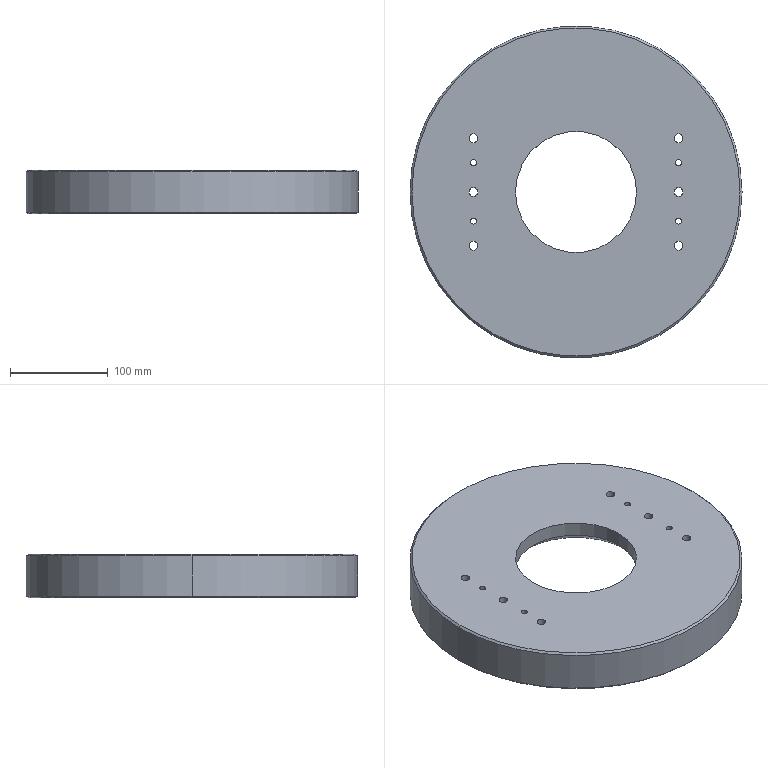NC program | NX | posted with a generic post | part box 340 x 340 x 45 mm
Lines 17007 to 17829 of 19805:
(ZLEVEL_PROFILE_COPY_COPY_1_COPY_COPY_2_COPY_1 , TOOL : D6R0.5)
N33964 T05 M6
N33966 G54
N33968 G17 G0 G90 X103.488 Y54.933 S7000 M3
N33970 G43 Z75. H5
N33972 Z34.929
N33974 G94 G1 X104.852 Y57.323 F3000.
N33976 G3 X104.85 Y57.923 R0.6
N33978 X101.682 Y63.181 R223.631
N33980 X-101.857 Y62.91 R119.714
N33982 G1 X-102.254 Y62.268
N33984 X-104.85 Y57.923
N33986 X-104.769 Z34.859
N33988 X-102.171 Y62.268
N33990 X-101.804 Y62.863
N33992 G2 X101.618 Y63.149 R119.647
N33994 X104.768 Y57.923 R223.465
N33996 G1 X104.686 Y57.924 Z34.788
N33998 X104.568 Y58.117
N34000 X102.832 Y61.035
N34002 G3 X-102.832 Y61.035 R119.581
N34004 G1 X-104.569 Y58.117
N34006 X-104.687 Y57.924
N34008 X-104.605 Z34.717
N34010 X-104.487 Y58.117
N34012 X-102.749 Y61.036
N34014 G2 X102.749 Y61.036 R119.51
N34016 G1 X104.486 Y58.117
N34018 X104.604 Y57.924
N34020 X104.521 Z34.646
N34022 X104.472 Y58.003
N34024 X102.666 Y61.037
N34026 G3 X-102.666 Y61.037 R119.439
N34028 G1 X-104.472 Y58.003
N34030 X-104.521 Y57.924
N34032 X-104.439 Z34.576
N34034 X-104.322 Y58.117
N34036 X-102.583 Y61.038
N34038 G2 X102.583 Y61.038 R119.369
N34040 G1 X104.322 Y58.117
N34042 X104.438 Y57.924
N34044 X104.357 Y57.925 Z34.505
N34046 X104.24 Y58.117
N34048 X102.501 Y61.037
N34050 G3 X-102.501 Y61.037 R119.298
N34052 G1 X-104.24 Y58.117
N34054 X-104.358 Y57.925
N34056 X-104.275 Y57.926 Z34.434
N34058 X-104.158 Y58.117
N34060 X-102.421 Y61.034
N34062 G2 X102.421 Y61.034 R119.227
N34064 G1 X104.158 Y58.117
N34066 X104.275 Y57.926
N34068 X104.192 Y57.925 Z34.364
N34070 X104.126 Y58.032
N34072 X102.34 Y61.031
N34074 G3 X-102.34 Y61.031 R119.157
N34076 G1 X-104.126 Y58.032
N34078 X-104.192 Y57.926
N34080 X-104.109 Y57.925 Z34.293
N34082 X-102.259 Y61.028
N34084 G2 X102.259 Y61.028 R119.086
N34086 G1 X104.109 Y57.925
N34088 X104.028 Y57.926 Z34.222
N34090 X103.911 Y58.117
N34092 X102.179 Y61.025
N34094 G3 X-102.179 Y61.025 R119.015
N34096 G1 X-103.911 Y58.117
N34098 X-104.028 Y57.927
N34100 X-103.946 Z34.151
N34102 X-103.829 Y58.117
N34104 X-102.1 Y61.019
N34106 G2 X102.1 Y61.019 R118.944
N34108 G1 X103.829 Y58.117
N34110 X103.946 Y57.927
N34112 X103.863 Z34.081
N34114 X103.78 Y58.061
N34116 X102.022 Y61.013
N34118 G3 X-102.022 Y61.013 R118.874
N34120 G1 X-103.78 Y58.061
N34122 X-103.863 Y57.927
N34124 X-103.779 Y57.926 Z34.01
N34126 X-101.943 Y61.006
N34128 G2 X101.943 Y61.006 R118.803
N34130 G1 X102.016 Y60.884
N34132 X103.779 Y57.926
N34134 X103.699 Y57.927 Z33.939
N34136 X103.583 Y58.117
N34138 X102.141 Y60.538
N34140 X101.865 Y60.999
N34142 G3 X-101.865 Y60.999 R118.732
N34144 G1 X-103.583 Y58.117
N34146 X-103.699 Y57.927
N34148 X-103.617 Y57.928 Z33.869
N34150 X-103.501 Y58.117
N34152 X-101.787 Y60.992
N34154 G2 X101.787 Y60.992 R118.662
N34156 G1 X102.058 Y60.538
N34158 X103.501 Y58.117
N34160 X103.617 Y57.928
N34162 X103.534 Z33.798
N34164 X103.434 Y58.091
N34166 X101.976 Y60.538
N34168 X101.71 Y60.982
N34170 G3 X-101.71 Y60.982 R118.591
N34172 G1 X-103.434 Y58.09
N34174 X-103.534 Y57.928
N34176 X-103.45 Y57.927 Z33.727
N34178 X-101.634 Y60.971
N34180 G2 X101.634 Y60.971 R118.52
N34182 G1 X101.894 Y60.538
N34184 X103.45 Y57.927
N34186 X103.371 Y57.926 Z33.657
N34188 X101.558 Y60.961
N34190 G3 X-101.558 Y60.961 R118.449
N34192 G1 X-103.371 Y57.926
N34194 X-103.291 Y57.925 Z33.586
N34196 X-101.482 Y60.95
N34198 G2 X101.482 Y60.95 R118.379
N34200 G1 X103.291 Y57.925
N34202 X103.21 Y57.923 Z33.515
N34204 X103.092 Y58.117
N34206 X101.406 Y60.939
N34208 G3 X-101.406 Y60.939 R118.308
N34210 G1 X-103.211 Y57.923
N34212 X-103.129 Y57.921 Z33.444
N34214 X-103.011 Y58.117
N34216 X-101.332 Y60.926
N34218 G2 X101.332 Y60.926 R118.237
N34220 G1 X103.129 Y57.921
N34222 X103.05 Y57.916 Z33.374
N34224 X101.257 Y60.912
N34226 G3 X-101.258 Y60.912 R118.167
N34228 G1 X-103.051 Y57.916
N34230 X-102.975 Y57.91 Z33.303
N34232 X-101.183 Y60.898
N34234 G2 X101.183 Y60.898 R118.096
N34236 G1 X102.974 Y57.91
N34238 X102.897 Y57.903 Z33.232
N34240 X101.109 Y60.884
N34242 G3 X-101.109 Y60.884 R118.025
N34244 G1 X-102.897 Y57.904
N34246 X-102.82 Y57.896 Z33.162
N34248 X-101.036 Y60.869
N34250 G2 X101.036 Y60.869 R117.954
N34252 G1 X102.819 Y57.896
N34254 X102.74 Y57.888 Z33.091
N34256 X101.013 Y60.77
N34258 X100.963 Y60.852
N34260 G3 X-100.963 Y60.852 R117.884
N34262 G1 X-102.741 Y57.889
N34264 X-102.668 Y57.878 Z33.02
N34266 X-100.891 Y60.835
N34268 G2 X100.891 Y60.835 R117.813
N34270 G1 X101.013 Y60.633
N34272 X102.396 Y58.328
N34274 X102.667 Y57.878
N34276 X102.592 Y57.867 Z32.949
N34278 X100.987 Y60.538
N34280 X100.819 Y60.818
N34282 G3 X-100.819 Y60.818 R117.742
N34284 G1 X-102.594 Y57.867
N34286 X-102.519 Y57.855 Z32.879
N34288 X-100.747 Y60.8
N34290 G2 X100.747 Y60.8 R117.672
N34292 G1 X100.905 Y60.538
N34294 X102.518 Y57.855
N34296 X102.443 Y57.843 Z32.808
N34298 X100.675 Y60.783
N34300 G3 X-100.675 Y60.783 R117.601
N34302 G1 X-102.444 Y57.844
N34304 X-102.37 Y57.831 Z32.737
N34306 X-100.604 Y60.763
N34308 G2 X100.604 Y60.763 R117.53
N34310 G1 X102.051 Y58.361
N34312 X102.369 Y57.83
N34314 X102.296 Y57.815 Z32.667
N34316 X100.534 Y60.742
N34318 G3 X-100.534 Y60.742 R117.459
N34320 G1 X-102.298 Y57.815
N34322 X-102.225 Y57.8 Z32.596
N34324 X-100.464 Y60.722
N34326 G2 X100.464 Y60.722 R117.389
N34328 G1 X102.224 Y57.8
N34330 X102.151 Y57.784 Z32.525
N34332 X100.701 Y60.193
N34334 X100.394 Y60.701
N34336 G3 X-100.394 Y60.701 R117.318
N34338 G1 X-102.153 Y57.785
N34340 X-102.081 Y57.769 Z32.454
N34342 X-100.324 Y60.68
N34344 G2 X100.324 Y60.68 R117.247
N34346 G1 X100.619 Y60.193
N34348 X102.079 Y57.769
N34350 X102.009 Y57.751 Z32.384
N34352 X100.255 Y60.657
N34354 G3 X-100.255 Y60.657 R117.177
N34356 G1 X-102.011 Y57.751
N34358 X-101.942 Y57.733 Z32.313
N34360 X-101.916 Y57.771
N34362 X-100.187 Y60.633
N34364 G2 X100.187 Y60.633 R117.106
N34366 G1 X101.94 Y57.732
N34368 X101.871 Y57.713 Z32.242
N34370 X101.832 Y57.771
N34372 X100.118 Y60.61
N34374 G3 X-100.118 Y60.61 R117.035
N34376 G1 X-101.834 Y57.771
N34378 X-101.873 Y57.714
N34380 X-101.803 Y57.695 Z32.172
N34382 X-101.753 Y57.771
N34384 X-100.05 Y60.586
N34386 G2 X100.05 Y60.586 R116.964
N34388 G1 X101.751 Y57.771
N34390 X101.802 Y57.694
N34392 X101.73 Y57.674 Z32.101
N34394 X101.705 Y57.712
N34396 X99.982 Y60.562
N34398 G3 X-99.982 Y60.562 R116.894
N34400 G1 X-101.705 Y57.715
N34402 X-101.732 Y57.674
N34404 X-101.663 Y57.652 Z32.03
N34406 X-101.589 Y57.771
N34408 X-99.915 Y60.537
N34410 G2 X99.915 Y60.537 R116.823
N34412 G1 X101.587 Y57.771
N34414 X101.662 Y57.651
N34416 X101.626 Y57.639 Z31.995
N34418 X101.596 Y57.629 Z31.959
N34420 X101.505 Y57.771
N34422 X99.848 Y60.51
N34424 G3 X-99.848 Y60.51 R116.752
N34426 G1 X-101.507 Y57.771
N34428 X-101.597 Y57.629
N34430 X-101.559 Y57.616 Z31.924
N34432 X-101.529 Y57.606 Z31.889
N34434 X-101.425 Y57.771
N34436 X-99.782 Y60.483
N34438 G2 X99.782 Y60.483 R116.682
N34440 G1 X101.423 Y57.771
N34442 X101.528 Y57.605
N34444 X101.49 Y57.592 Z31.853
N34446 X101.46 Y57.581 Z31.818
N34448 X101.359 Y57.742
N34450 X99.715 Y60.456
N34452 G3 X-99.715 Y60.456 R116.611
N34454 G1 X-101.359 Y57.745
N34456 X-101.461 Y57.582
N34458 X-101.424 Y57.569 Z31.783
N34460 X-101.392 Y57.557 Z31.747
N34462 X-101.359 Y57.609
N34464 X-99.649 Y60.429
N34466 G2 X99.649 Y60.429 R116.54
N34468 G1 X101.39 Y57.556
N34470 X101.356 Y57.543 Z31.712
N34472 X101.323 Y57.531 Z31.677
N34474 X99.583 Y60.401
N34476 G3 X-99.583 Y60.401 R116.469
N34478 G1 X-101.325 Y57.531
N34480 X-101.291 Y57.517 Z31.641
N34482 X-101.26 Y57.504 Z31.606
N34484 X-99.519 Y60.371
N34486 G2 X99.519 Y60.371 R116.399
N34488 G1 X101.258 Y57.503
N34490 X101.224 Y57.489 Z31.571
N34492 X101.192 Y57.476 Z31.535
N34494 X99.454 Y60.341
N34496 G3 X-99.454 Y60.341 R116.328
N34498 G1 X-101.194 Y57.477
N34500 X-101.16 Y57.463 Z31.5
N34502 X-101.127 Y57.449 Z31.464
N34504 X-99.39 Y60.312
N34506 G2 X99.39 Y60.312 R116.257
N34508 G1 X101.126 Y57.448
N34510 X101.093 Y57.434 Z31.429
N34512 X101.06 Y57.421 Z31.394
N34514 X99.325 Y60.282
N34516 G3 X-99.325 Y60.282 R116.187
N34518 G1 X-101.062 Y57.421
N34520 X-101.029 Y57.406 Z31.358
N34522 X-100.998 Y57.391 Z31.323
N34524 X-99.261 Y60.252
N34526 G2 X99.261 Y60.252 R116.116
N34528 G1 X100.997 Y57.391
N34530 X100.964 Y57.375 Z31.288
N34532 X100.935 Y57.36 Z31.252
N34534 X100.892 Y57.425
N34536 X99.198 Y60.219
N34538 G3 X-99.198 Y60.219 R116.045
N34540 G1 X-100.894 Y57.425
N34542 X-100.936 Y57.361
N34544 X-100.902 Y57.344 Z31.217
N34546 X-100.874 Y57.33 Z31.182
N34548 X-100.812 Y57.425
N34550 X-99.135 Y60.186
N34552 G2 X99.135 Y60.186 R115.975
N34554 G1 X100.81 Y57.425
N34556 X100.873 Y57.33
N34558 X100.837 Y57.312 Z31.146
N34560 X100.81 Y57.298 Z31.111
N34562 X100.728 Y57.425
N34564 X99.072 Y60.153
N34566 G3 X-99.072 Y60.153 R115.904
N34568 G1 X-100.729 Y57.425
N34570 X-100.811 Y57.299
N34572 X-100.776 Y57.281 Z31.076
N34574 X-100.747 Y57.267 Z31.04
N34576 X-100.667 Y57.392
N34578 X-99.009 Y60.121
N34580 G2 X99.009 Y60.121 R115.833
N34582 G1 X100.667 Y57.389
N34584 X100.746 Y57.267
N34586 X100.711 Y57.249 Z31.005
N34588 X100.68 Y57.233 Z30.969
N34590 X98.946 Y60.088
N34592 G3 X-98.946 Y60.088 R115.762
N34594 G1 X-100.681 Y57.234
N34596 X-100.65 Y57.217 Z30.934
N34598 X-100.62 Y57.201 Z30.899
N34600 X-100.482 Y57.425
N34602 X-98.885 Y60.052
N34604 G2 X98.885 Y60.052 R115.692
N34606 G1 X100.48 Y57.425
N34608 X100.619 Y57.2
N34610 X100.587 Y57.181 Z30.863
N34612 X100.558 Y57.165 Z30.828
N34614 X100.398 Y57.425
N34616 X98.824 Y60.017
N34618 G3 X-98.824 Y60.017 R115.621
N34620 G1 X-100.399 Y57.425
N34622 X-100.559 Y57.166
N34624 X-100.527 Y57.147 Z30.793
N34626 X-100.497 Y57.13 Z30.757
N34628 X-98.763 Y59.981
N34630 G2 X98.763 Y59.981 R115.55
N34632 G1 X100.496 Y57.13
N34634 X100.464 Y57.112 Z30.722
N34636 X100.434 Y57.094 Z30.687
N34638 X98.702 Y59.945
N34640 G3 X-98.702 Y59.945 R115.48
N34642 G1 X-100.435 Y57.095
N34644 X-100.404 Y57.077 Z30.651
N34646 X-100.375 Y57.06 Z30.616
N34648 X-100.361 Y57.079
N34650 X-98.641 Y59.909
N34652 G2 X98.641 Y59.909 R115.409
N34654 G1 X100.36 Y57.079
N34656 X100.374 Y57.06
N34658 X100.342 Y57.04 Z30.581
N34660 X100.313 Y57.022 Z30.545
N34662 X98.386 Y60.193
N34664 G3 X-98.386 Y60.193 R115.338
N34666 G1 X-100.313 Y57.023
N34668 X-100.283 Y57.003 Z30.51
N34670 X-100.256 Y56.985 Z30.475
N34672 X-100.196 Y57.079
N34674 X-98.514 Y59.847
N34676 G2 X98.514 Y59.847 R115.267
N34678 G1 X100.195 Y57.079
N34680 X100.255 Y56.985
N34682 X100.224 Y56.964 Z30.439
N34684 X100.198 Y56.947 Z30.404
N34686 X100.112 Y57.079
N34688 X98.463 Y59.795
N34690 G3 X-98.463 Y59.795 R115.197
N34692 G1 X-100.113 Y57.079
N34694 X-100.198 Y56.947
N34696 X-100.165 Y56.925 Z30.368
N34698 X-100.139 Y56.908 Z30.333
N34700 X-100.03 Y57.079
N34702 X-98.403 Y59.756
N34704 G2 X98.403 Y59.756 R115.126
N34706 G1 X100.03 Y57.079
N34708 X100.139 Y56.908
N34710 X100.106 Y56.886 Z30.298
N34712 X100.079 Y56.869 Z30.262
N34714 X99.975 Y57.033
N34716 X98.344 Y59.717
N34718 G3 X-98.344 Y59.717 R115.055
N34720 G1 X-99.975 Y57.034
N34722 X-100.079 Y56.869
N34724 X-100.047 Y56.848 Z30.227
N34726 X-100.018 Y56.829 Z30.192
N34728 X-99.975 Y56.898
N34730 X-98.286 Y59.677
N34732 G2 X98.286 Y59.677 R114.985
N34734 G1 X99.975 Y56.897
N34736 X100.018 Y56.829
N34738 X99.987 Y56.809 Z30.156
N34740 X99.958 Y56.789 Z30.121
N34742 X98.228 Y59.636
N34744 G3 X-98.228 Y59.636 R114.914
N34746 G1 X-99.958 Y56.789
N34748 X-99.929 Y56.769 Z30.086
N34750 X-99.9 Y56.749 Z30.05
N34752 X-98.17 Y59.595
N34754 G2 X98.17 Y59.595 R114.843
N34756 G1 X99.899 Y56.749
N34758 X99.87 Y56.729 Z30.015
N34760 X99.842 Y56.71 Z29.98
N34762 X99.826 Y56.733
N34764 X98.113 Y59.553
N34766 G3 X-98.113 Y59.553 R114.772
N34768 G1 X-99.826 Y56.733
N34770 X-99.842 Y56.71
N34772 X-99.811 Y56.69 Z29.944
N34774 X-99.785 Y56.672 Z29.909
N34776 X-99.744 Y56.733
N34778 X-98.056 Y59.511
N34780 G2 X98.056 Y59.511 R114.702
N34782 G1 X99.744 Y56.733
N34784 X99.785 Y56.672
N34786 X99.753 Y56.65 Z29.873
N34788 X99.728 Y56.632 Z29.838
N34790 G3 X94.632 Y64.69 R167.72
N34792 X-97.334 Y60.538 R114.627
N34794 G1 X-97.55 Y60.193
N34796 X-97.766 Y59.847
N34798 X-97.899 Y59.632
N34800 X-99.661 Y56.733
N34802 X-99.727 Y56.632
N34804 X-99.694 Y56.61 Z29.803
N34806 X-99.667 Y56.591 Z29.767
N34808 X-99.629 Y56.649
N34810 X-97.896 Y59.501
N34812 X-97.463 Y60.203
N34814 G2 X96.144 Y62.272 R114.545
N34816 X99.667 Y56.592 R171.346
N34818 G1 X99.637 Y56.571 Z29.734
N34820 X99.61 Y56.553 Z29.701
N34822 G3 X96.061 Y62.278 R167.554
N34824 X-97.331 Y60.287 R114.48
N34826 G1 X-97.818 Y59.501
N34828 X-99.61 Y56.553
N34830 X-99.582 Y56.533 Z29.667
N34832 X-99.556 Y56.516 Z29.634
N34834 X-99.421 Y56.733
N34836 X-97.775 Y59.442
N34838 G2 X96.026 Y62.21 R114.415
N34840 X99.556 Y56.516 R169.986
N34842 G1 X99.527 Y56.496 Z29.6
N34844 X99.501 Y56.478 Z29.567
N34846 G3 X95.966 Y62.18 R169.264
N34848 X-97.713 Y59.414 R114.349
N34850 G1 X-99.343 Y56.733
N34852 X-99.5 Y56.478
N34854 X-99.471 Y56.458 Z29.533
N34856 X-99.444 Y56.44 Z29.5
N34858 X-97.582 Y59.501
N34860 G2 X96.064 Y61.922 R114.297
N34862 X99.445 Y56.44 R275.708
N34864 X99.455 Y55.841 R0.6
N34866 G1 X98.123 Y53.438
N34868 G0 Z75.
N34870 X-104.091 Y53.788
N34872 Z34.929
N34874 G1 X-106.825 Y53.556
N34876 G3 X-107.317 Y53.213 R0.6
N34878 X-110.176 Y46.819 R190.395
N34880 X-109.359 Y-48.705 R119.669
N34882 G1 X-108.865 Y-49.814
N34884 X-107.318 Y-53.213
N34886 X-107.271 Y-53.145 Z34.859
N34888 X-108.991 Y-49.349
N34890 G2 X-110.126 Y46.756 R119.588
N34892 X-107.271 Y53.145 R187.962
N34894 G1 X-107.225 Y53.077 Z34.788
N34896 X-107.24 Y53.04
N34898 X-108.71 Y49.814
N34900 X-108.726 Y49.781
N34902 G3 X-108.726 Y-49.781 R119.581
N34904 G1 X-107.24 Y-53.041
N34906 X-107.225 Y-53.077
N34908 X-107.181 Y-53.011 Z34.717
N34910 X-107.214 Y-52.928
N34912 X-108.68 Y-49.713
N34914 G2 X-108.68 Y49.713 R119.51
N34916 G1 X-107.213 Y52.928
N34918 X-107.181 Y53.01
N34920 X-107.131 Y52.941 Z34.646
N34922 X-108.633 Y49.644
N34924 G3 X-108.633 Y-49.644 R119.439
N34926 G1 X-107.131 Y-52.941
N34928 X-107.085 Y-52.874 Z34.576
N34930 X-107.216 Y-52.582
N34932 X-108.587 Y-49.575
N34934 G2 X-108.587 Y49.575 R119.369
N34936 G1 X-107.216 Y52.582
N34938 X-107.085 Y52.874
N34940 X-107.039 Y52.807 Z34.505
N34942 X-107.138 Y52.582
N34944 X-108.54 Y49.508
N34946 G3 X-108.54 Y-49.508 R119.298
N34948 G1 X-107.138 Y-52.582
N34950 X-107.04 Y-52.807
N34952 X-106.993 Y-52.739 Z34.434
N34954 X-107.061 Y-52.582
N34956 X-108.492 Y-49.444
N34958 G2 X-108.492 Y49.444 R119.227
N34960 G1 X-107.061 Y52.582
N34962 X-106.993 Y52.739
N34964 X-106.945 Y52.671 Z34.364
N34966 X-106.983 Y52.582
N34968 X-108.443 Y49.379
N34970 G3 X-108.443 Y-49.379 R119.157
N34972 G1 X-106.983 Y-52.582
N34974 X-106.945 Y-52.671
N34976 X-106.897 Y-52.602 Z34.293
N34978 X-108.395 Y-49.315
N34980 G2 X-108.395 Y49.315 R119.086
N34982 G1 X-106.896 Y52.602
N34984 X-106.851 Y52.535 Z34.222
N34986 X-106.894 Y52.438
N34988 X-108.347 Y49.25
N34990 G3 X-108.347 Y-49.25 R119.015
N34992 G1 X-106.894 Y-52.438
N34994 X-106.851 Y-52.535
N34996 X-106.807 Y-52.468 Z34.151
N34998 X-106.894 Y-52.268
N35000 X-108.297 Y-49.189
N35002 G2 X-108.297 Y49.189 R118.944
N35004 G1 X-106.894 Y52.267
N35006 X-106.807 Y52.468
N35008 X-106.761 Y52.401 Z34.081
N35010 X-106.83 Y52.236
N35012 X-108.247 Y49.128
N35014 G3 X-108.247 Y-49.128 R118.874
N35016 G1 X-106.83 Y-52.236
N35018 X-106.761 Y-52.401
N35020 X-106.714 Y-52.332 Z34.01
N35022 X-106.753 Y-52.236
N35024 X-108.197 Y-49.068
N35026 G2 X-108.197 Y49.068 R118.803
N35028 G1 X-106.753 Y52.236
N35030 X-106.713 Y52.332
N35032 X-106.664 Y52.263 Z33.939
N35034 X-108.146 Y49.007
N35036 G3 X-108.146 Y-49.007 R118.732
N35038 G1 X-106.664 Y-52.264
N35040 X-106.617 Y-52.195 Z33.869
N35042 X-108.096 Y-48.947
N35044 G2 X-108.096 Y48.947 R118.662
N35046 G1 X-106.617 Y52.195
N35048 X-106.57 Y52.128 Z33.798
N35050 X-108.044 Y48.89
N35052 G3 X-108.044 Y-48.89 R118.591
N35054 G1 X-106.57 Y-52.128
N35056 X-106.525 Y-52.061 Z33.727
N35058 X-107.992 Y-48.833
N35060 G2 X-107.992 Y48.833 R118.52
N35062 G1 X-106.548 Y52.005
N35064 X-106.525 Y52.061
N35066 X-106.48 Y51.996 Z33.657
N35068 X-106.523 Y51.89
N35070 X-107.784 Y49.123
N35072 X-107.942 Y48.773
N35074 G3 X-107.942 Y-48.773 R118.449
N35076 G1 X-106.523 Y-51.89
N35078 X-106.48 Y-51.996
N35080 X-106.431 Y-51.928 Z33.586
N35082 X-106.604 Y-51.544
N35084 X-107.888 Y-48.72
N35086 G2 X-107.888 Y48.72 R118.379
N35088 G1 X-106.431 Y51.928
N35090 X-106.382 Y51.863 Z33.515
N35092 X-107.836 Y48.664
N35094 G3 X-107.836 Y-48.664 R118.308
N35096 G1 X-106.382 Y-51.863
N35098 X-106.335 Y-51.802 Z33.444
N35100 X-107.783 Y-48.61
N35102 G2 X-107.783 Y48.61 R118.237
N35104 G1 X-106.335 Y51.802
N35106 X-106.287 Y51.74 Z33.374
N35108 X-107.729 Y48.558
N35110 G3 X-107.729 Y-48.558 R118.167
N35112 G1 X-106.287 Y-51.74
N35114 X-106.238 Y-51.677 Z33.303
N35116 X-107.675 Y-48.505
N35118 G2 X-107.675 Y48.505 R118.096
N35120 G1 X-106.238 Y51.677
N35122 X-106.189 Y51.616 Z33.232
N35124 X-107.621 Y48.452
N35126 G3 X-107.621 Y-48.452 R118.025
N35128 G1 X-106.189 Y-51.616
N35130 X-106.139 Y-51.556 Z33.162
N35132 X-107.568 Y-48.399
N35134 G2 X-107.568 Y48.399 R117.954
N35136 G1 X-106.139 Y51.556
N35138 X-106.088 Y51.5 Z33.091
N35140 X-107.512 Y48.349
N35142 G3 X-107.512 Y-48.349 R117.884
N35144 G1 X-106.088 Y-51.5
N35146 X-106.038 Y-51.445 Z33.02
N35148 X-107.457 Y-48.3
N35150 G2 X-107.457 Y48.3 R117.813
N35152 G1 X-106.038 Y51.445
N35154 X-105.987 Y51.39 Z32.949
N35156 X-106.07 Y51.198
N35158 X-107.402 Y48.251
N35160 G3 X-107.402 Y-48.251 R117.742
N35162 G1 X-106.07 Y-51.198
N35164 X-105.987 Y-51.39
N35166 X-105.935 Y-51.335 Z32.879
N35168 X-105.994 Y-51.198
N35170 X-107.346 Y-48.201
N35172 G2 X-107.346 Y48.201 R117.672
N35174 G1 X-105.994 Y51.198
N35176 X-105.935 Y51.335
N35178 X-105.882 Y51.279 Z32.808
N35180 X-107.291 Y48.152
N35182 G3 X-107.291 Y-48.152 R117.601
N35184 G1 X-106.074 Y-50.852
N35186 X-105.882 Y-51.279
N35188 X-105.83 Y-51.225 Z32.737
N35190 X-107.235 Y-48.105
N35192 G2 X-107.235 Y48.105 R117.53
N35194 G1 X-105.83 Y51.225
N35196 X-105.775 Y51.174 Z32.667
N35198 X-107.177 Y48.06
N35200 G3 X-107.177 Y-48.06 R117.459
N35202 G1 X-105.92 Y-50.852
N35204 X-105.775 Y-51.174
N35206 X-105.723 Y-51.125 Z32.596
N35208 X-105.843 Y-50.852
N35210 X-107.12 Y-48.014
N35212 G2 X-107.12 Y48.014 R117.389
N35214 G1 X-107.089 Y48.085
N35216 X-105.843 Y50.852
N35218 X-105.723 Y51.125
N35220 X-105.669 Y51.075 Z32.525
N35222 X-105.766 Y50.852
N35224 X-107.063 Y47.968
N35226 G3 X-107.063 Y-47.968 R117.318
N35228 G1 X-105.766 Y-50.852
N35230 X-105.669 Y-51.075
N35232 X-105.615 Y-51.026 Z32.454
N35234 X-105.69 Y-50.852
N35236 X-107.007 Y-47.922
N35238 G2 X-107.007 Y47.922 R117.247
N35240 G1 X-105.69 Y50.852
N35242 X-105.615 Y51.026
N35244 X-105.56 Y50.975 Z32.384
N35246 X-105.613 Y50.852
N35248 X-106.949 Y47.878
N35250 G3 X-106.949 Y-47.878 R117.177
N35252 G1 X-105.613 Y-50.852
N35254 X-105.56 Y-50.976
N35256 X-105.504 Y-50.926 Z32.313
N35258 X-106.89 Y-47.836
N35260 G2 X-106.89 Y47.836 R117.106
N35262 G1 X-105.504 Y50.926
N35264 X-105.449 Y50.88 Z32.242
N35266 X-105.459 Y50.852
N35268 X-106.832 Y47.793
N35270 G3 X-106.832 Y-47.793 R117.035
N35272 G1 X-105.459 Y-50.852
N35274 X-105.449 Y-50.88
N35276 X-105.391 Y-50.835 Z32.172
N35278 X-106.773 Y-47.751
N35280 G2 X-106.773 Y47.751 R116.964
N35282 G1 X-105.391 Y50.835
N35284 X-105.362 Y50.813 Z32.136
N35286 X-105.335 Y50.791 Z32.101
N35288 X-106.715 Y47.709
N35290 G3 X-106.715 Y-47.709 R116.894
N35292 G1 X-105.335 Y-50.791
N35294 X-105.305 Y-50.768 Z32.066
N35296 X-105.278 Y-50.748 Z32.03
N35298 X-105.384 Y-50.506
N35300 X-106.656 Y-47.667
N35302 G2 X-106.656 Y47.667 R116.823
N35304 G1 X-105.278 Y50.748
N35306 X-105.248 Y50.724 Z31.995
N35308 X-105.221 Y50.704 Z31.959
N35310 X-105.307 Y50.506
N35312 X-106.596 Y47.628
N35314 G3 X-106.596 Y-47.628 R116.752
N35316 G1 X-105.307 Y-50.506
N35318 X-105.221 Y-50.704
N35320 X-105.19 Y-50.681 Z31.924
N35322 X-105.162 Y-50.659 Z31.889
N35324 X-106.536 Y-47.589
N35326 G2 X-106.536 Y47.589 R116.682
N35328 G1 X-105.162 Y50.659
N35330 X-105.132 Y50.638 Z31.853
N35332 X-105.107 Y50.62 Z31.818
N35334 X-105.153 Y50.506
N35336 X-106.476 Y47.55
N35338 G3 X-106.476 Y-47.55 R116.611
N35340 G1 X-105.153 Y-50.506
N35342 X-105.107 Y-50.62
N35344 X-105.074 Y-50.597 Z31.783
N35346 X-105.047 Y-50.579 Z31.747
N35348 X-105.076 Y-50.506
N35350 X-106.416 Y-47.511
N35352 G2 X-106.416 Y47.511 R116.54
N35354 G1 X-105.076 Y50.506
N35356 X-105.047 Y50.579
N35358 X-105.015 Y50.557 Z31.712
N35360 X-104.987 Y50.538 Z31.677
N35362 X-104.999 Y50.506
N35364 X-106.356 Y47.472
N35366 G3 X-106.356 Y-47.472 R116.469
N35368 G1 X-104.999 Y-50.506
N35370 X-104.987 Y-50.538
N35372 X-104.956 Y-50.517 Z31.641
N35374 X-104.927 Y-50.497 Z31.606
N35376 X-106.295 Y-47.436
N35378 G2 X-106.295 Y47.436 R116.399
N35380 G1 X-104.927 Y50.497
N35382 X-104.897 Y50.477 Z31.571
N35384 X-104.867 Y50.458 Z31.535
N35386 X-106.233 Y47.399
N35388 G3 X-106.233 Y-47.399 R116.328
N35390 G1 X-104.867 Y-50.458
N35392 X-104.837 Y-50.439 Z31.5
N35394 X-104.807 Y-50.42 Z31.464
N35396 X-106.172 Y-47.364
N35398 G2 X-106.172 Y47.364 R116.257
N35400 G1 X-104.807 Y50.42
N35402 X-104.776 Y50.402 Z31.429
N35404 X-104.748 Y50.385 Z31.394
N35406 X-104.818 Y50.222
N35408 X-106.11 Y47.328
N35410 G3 X-106.11 Y-47.328 R116.187
N35412 G1 X-104.818 Y-50.222
N35414 X-104.748 Y-50.385
N35416 X-104.715 Y-50.366 Z31.358
N35418 X-104.688 Y-50.35 Z31.323
N35420 X-104.768 Y-50.16
N35422 X-106.049 Y-47.292
N35424 G2 X-106.049 Y47.292 R116.116
N35426 G1 X-104.769 Y50.16
N35428 X-104.688 Y50.35
N35430 X-104.654 Y50.331 Z31.288
N35432 X-104.626 Y50.315 Z31.252
N35434 X-104.691 Y50.16
N35436 X-105.987 Y47.258
N35438 G3 X-105.987 Y-47.258 R116.045
N35440 G1 X-104.691 Y-50.16
N35442 X-104.626 Y-50.315
N35444 X-104.592 Y-50.296 Z31.217
N35446 X-104.565 Y-50.28 Z31.182
N35448 X-104.614 Y-50.16
N35450 X-105.924 Y-47.226
N35452 G2 X-105.924 Y47.226 R115.975
N35454 G1 X-104.614 Y50.16
N35456 X-104.565 Y50.28
N35458 X-104.531 Y50.26 Z31.146
N35460 X-104.502 Y50.244 Z31.111
N35462 X-104.537 Y50.16
N35464 X-105.861 Y47.193
N35466 G3 X-105.861 Y-47.193 R115.904
N35468 G1 X-104.537 Y-50.16
N35470 X-104.502 Y-50.244
N35472 X-104.469 Y-50.226 Z31.076
N35474 X-104.441 Y-50.21 Z31.04
N35476 X-104.46 Y-50.16
N35478 X-105.798 Y-47.16
N35480 G2 X-105.798 Y47.16 R115.833
N35482 G1 X-104.46 Y50.16
N35484 X-104.441 Y50.21
N35486 X-104.407 Y50.193 Z31.005
N35488 X-104.376 Y50.177 Z30.969
N35490 X-105.735 Y47.128
N35492 G3 X-105.735 Y-47.128 R115.762
N35494 G1 X-104.376 Y-50.177
N35496 X-104.344 Y-50.161 Z30.934
N35498 X-104.313 Y-50.145 Z30.899
N35500 X-105.672 Y-47.096
N35502 G2 X-105.672 Y47.096 R115.692
N35504 G1 X-104.313 Y50.145
N35506 X-104.28 Y50.13 Z30.863
N35508 X-104.249 Y50.115 Z30.828
N35510 X-105.608 Y47.067
N35512 G3 X-105.608 Y-47.067 R115.621
N35514 G1 X-104.249 Y-50.115
N35516 X-104.217 Y-50.099 Z30.793
N35518 X-104.186 Y-50.085 Z30.757
N35520 X-105.543 Y-47.037
N35522 G2 X-105.543 Y47.037 R115.55
N35524 G1 X-104.186 Y50.085
N35526 X-104.153 Y50.069 Z30.722
N35528 X-104.122 Y50.054 Z30.687
N35530 X-105.479 Y47.008
N35532 G3 X-105.479 Y-47.008 R115.48
N35534 G1 X-104.122 Y-50.054
N35536 X-104.089 Y-50.04 Z30.651
N35538 X-104.059 Y-50.027 Z30.616
N35540 X-104.126 Y-49.87
N35542 X-105.415 Y-46.978
N35544 G2 X-105.415 Y46.978 R115.409
N35546 G1 X-104.126 Y49.87
N35548 X-104.059 Y50.027
N35550 X-104.024 Y50.012 Z30.581
N35552 X-103.995 Y50. Z30.545
N35554 X-104.074 Y49.814
N35556 X-105.35 Y46.949
N35558 G3 X-105.35 Y-46.949 R115.338
N35560 G1 X-104.074 Y-49.814
N35562 X-103.995 Y-50.
N35564 X-103.959 Y-49.985 Z30.51
N35566 X-103.93 Y-49.972 Z30.475
N35568 X-103.996 Y-49.814
N35570 X-105.285 Y-46.922
N35572 G2 X-105.285 Y46.922 R115.267
N35574 G1 X-103.996 Y49.814
N35576 X-103.93 Y49.972
N35578 X-103.894 Y49.957 Z30.439
N35580 X-103.865 Y49.944 Z30.404
N35582 X-103.919 Y49.814
N35584 X-105.219 Y46.896
N35586 G3 X-105.219 Y-46.896 R115.197
N35588 G1 X-103.919 Y-49.814
N35590 X-103.865 Y-49.944
N35592 X-103.829 Y-49.929 Z30.368
N35594 X-103.798 Y-49.916 Z30.333
N35596 X-103.842 Y-49.814
N35598 X-105.164 Y-46.846
N35600 G2 X-105.164 Y46.846 R115.126
N35602 G1 X-103.798 Y49.916